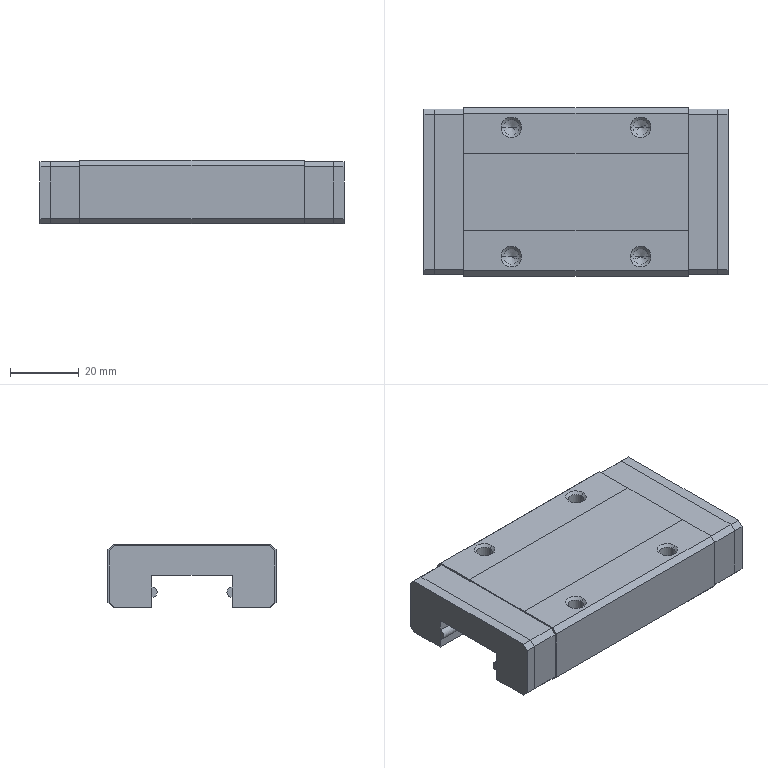Part | STEP file | 1 solid | 79 faces | box 88.2 x 48.75 x 18.375 mm | volume 58847 mm3 | plane 52 | cone 16 | cylinder 11 | commonest cylinder face diameters 4.5 x8 3 x3